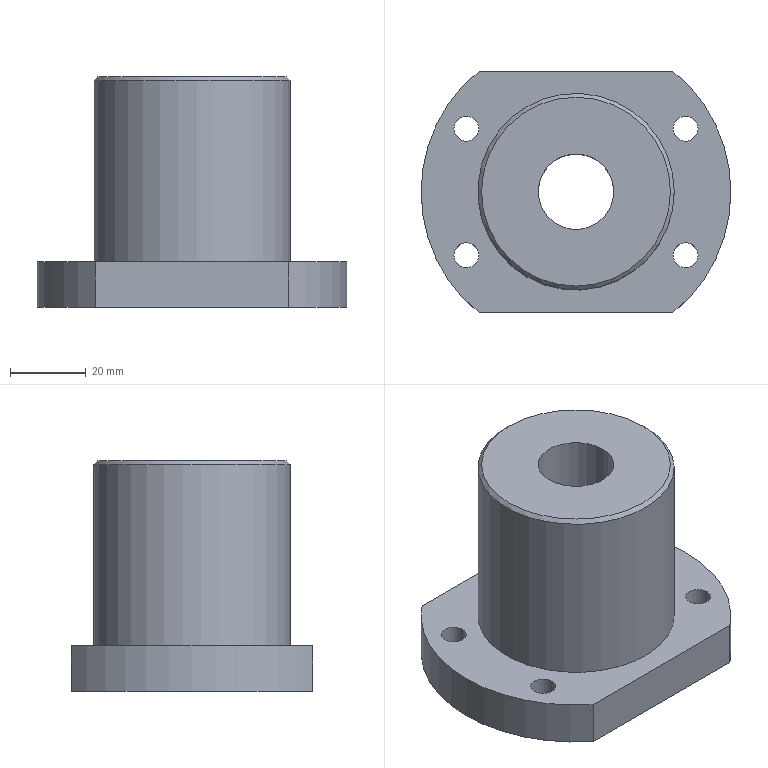Part | NX | 1 solid | 14 faces | box 82 x 64 x 61 mm | volume 138987 mm3 | cylinder 8 | plane 5 | cone 1 | commonest cylinder face diameters 6.6 x4 82 x2 20 x1 52 x1
STEP:
#1=CARTESIAN_POINT('',(32.312,16.75,12.));
#2=VERTEX_POINT('',#1);
#3=CARTESIAN_POINT('',(29.012,16.75,12.));
#4=DIRECTION('',(0.,0.,1.));
#5=DIRECTION('',(1.,0.,0.));
#6=AXIS2_PLACEMENT_3D('',#3,#4,#5);
#7=CIRCLE('',#6,3.3);
#8=EDGE_CURVE('',#2,#2,#7,.T.);
#9=ORIENTED_EDGE('',*,*,#8,.F.);
#10=EDGE_LOOP('',(#9));
#11=FACE_BOUND('',#10,.T.);
#12=CARTESIAN_POINT('',(-25.712,16.75,12.));
#13=VERTEX_POINT('',#12);
#14=CARTESIAN_POINT('',(-29.012,16.75,12.));
#15=DIRECTION('',(0.,0.,1.));
#16=DIRECTION('',(1.,0.,0.));
#17=AXIS2_PLACEMENT_3D('',#14,#15,#16);
#18=CIRCLE('',#17,3.3);
#19=EDGE_CURVE('',#13,#13,#18,.T.);
#20=ORIENTED_EDGE('',*,*,#19,.F.);
#21=EDGE_LOOP('',(#20));
#22=FACE_BOUND('',#21,.T.);
#23=CARTESIAN_POINT('',(32.312,-16.75,12.));
#24=VERTEX_POINT('',#23);
#25=CARTESIAN_POINT('',(29.012,-16.75,12.));
#26=DIRECTION('',(0.,0.,1.));
#27=DIRECTION('',(1.,0.,0.));
#28=AXIS2_PLACEMENT_3D('',#25,#26,#27);
#29=CIRCLE('',#28,3.3);
#30=EDGE_CURVE('',#24,#24,#29,.T.);
#31=ORIENTED_EDGE('',*,*,#30,.F.);
#32=EDGE_LOOP('',(#31));
#33=FACE_BOUND('',#32,.T.);
#34=CARTESIAN_POINT('',(-25.712,-16.75,12.));
#35=VERTEX_POINT('',#34);
#36=CARTESIAN_POINT('',(-29.012,-16.75,12.));
#37=DIRECTION('',(0.,0.,1.));
#38=DIRECTION('',(1.,0.,0.));
#39=AXIS2_PLACEMENT_3D('',#36,#37,#38);
#40=CIRCLE('',#39,3.3);
#41=EDGE_CURVE('',#35,#35,#40,.T.);
#42=ORIENTED_EDGE('',*,*,#41,.F.);
#43=EDGE_LOOP('',(#42));
#44=FACE_BOUND('',#43,.T.);
#45=CARTESIAN_POINT('',(26.,0.,12.));
#46=VERTEX_POINT('',#45);
#47=CARTESIAN_POINT('',(0.,0.,12.));
#48=DIRECTION('',(0.,0.,1.));
#49=DIRECTION('',(1.,0.,0.));
#50=AXIS2_PLACEMENT_3D('',#47,#48,#49);
#51=CIRCLE('',#50,26.);
#52=EDGE_CURVE('',#46,#46,#51,.T.);
#53=ORIENTED_EDGE('',*,*,#52,.F.);
#54=EDGE_LOOP('',(#53));
#55=FACE_BOUND('',#54,.T.);
#56=CARTESIAN_POINT('',(-25.632,32.,12.));
#57=VERTEX_POINT('',#56);
#58=CARTESIAN_POINT('',(-25.632,-32.,12.));
#59=VERTEX_POINT('',#58);
#60=CARTESIAN_POINT('',(0.,0.,12.));
#61=DIRECTION('',(0.,0.,1.));
#62=DIRECTION('',(1.,0.,0.));
#63=AXIS2_PLACEMENT_3D('',#60,#61,#62);
#64=CIRCLE('',#63,41.);
#65=EDGE_CURVE('',#57,#59,#64,.T.);
#66=ORIENTED_EDGE('',*,*,#65,.T.);
#67=CARTESIAN_POINT('',(25.632,-32.,12.));
#68=VERTEX_POINT('',#67);
#69=CARTESIAN_POINT('',(0.,-32.,12.));
#70=DIRECTION('',(1.,0.,0.));
#71=VECTOR('',#70,1000.);
#72=LINE('',#69,#71);
#73=EDGE_CURVE('',#59,#68,#72,.T.);
#74=ORIENTED_EDGE('',*,*,#73,.T.);
#75=CARTESIAN_POINT('',(25.632,32.,12.));
#76=VERTEX_POINT('',#75);
#77=CARTESIAN_POINT('',(0.,0.,12.));
#78=DIRECTION('',(0.,0.,1.));
#79=DIRECTION('',(1.,0.,0.));
#80=AXIS2_PLACEMENT_3D('',#77,#78,#79);
#81=CIRCLE('',#80,41.);
#82=EDGE_CURVE('',#68,#76,#81,.T.);
#83=ORIENTED_EDGE('',*,*,#82,.T.);
#84=CARTESIAN_POINT('',(0.,32.,12.));
#85=DIRECTION('',(-1.,0.,0.));
#86=VECTOR('',#85,1000.);
#87=LINE('',#84,#86);
#88=EDGE_CURVE('',#76,#57,#87,.T.);
#89=ORIENTED_EDGE('',*,*,#88,.T.);
#90=EDGE_LOOP('',(#66,#74,#83,#89));
#91=FACE_BOUND('',#90,.T.);
#92=CARTESIAN_POINT('',(0.,0.,12.));
#93=DIRECTION('',(0.,0.,1.));
#94=DIRECTION('',(1.,0.,0.));
#95=AXIS2_PLACEMENT_3D('',#92,#93,#94);
#96=PLANE('',#95);
#97=ADVANCED_FACE('',(#11,#22,#33,#44,#55,#91),#96,.T.);
#98=CARTESIAN_POINT('',(-25.632,-32.,0.));
#99=VERTEX_POINT('',#98);
#100=CARTESIAN_POINT('',(-25.632,-32.,12.));
#101=DIRECTION('',(0.,0.,-1.));
#102=VECTOR('',#101,1000.);
#103=LINE('',#100,#102);
#104=EDGE_CURVE('',#59,#99,#103,.T.);
#105=ORIENTED_EDGE('',*,*,#104,.F.);
#106=ORIENTED_EDGE('',*,*,#65,.F.);
#107=CARTESIAN_POINT('',(-25.632,32.,0.));
#108=VERTEX_POINT('',#107);
#109=CARTESIAN_POINT('',(-25.632,32.,12.));
#110=DIRECTION('',(0.,0.,-1.));
#111=VECTOR('',#110,1000.);
#112=LINE('',#109,#111);
#113=EDGE_CURVE('',#108,#57,#112,.F.);
#114=ORIENTED_EDGE('',*,*,#113,.F.);
#115=CARTESIAN_POINT('',(0.,0.,0.));
#116=DIRECTION('',(0.,0.,1.));
#117=DIRECTION('',(1.,0.,0.));
#118=AXIS2_PLACEMENT_3D('',#115,#116,#117);
#119=CIRCLE('',#118,41.);
#120=EDGE_CURVE('',#108,#99,#119,.T.);
#121=ORIENTED_EDGE('',*,*,#120,.T.);
#122=EDGE_LOOP('',(#105,#106,#114,#121));
#123=FACE_BOUND('',#122,.T.);
#124=CARTESIAN_POINT('',(0.,0.,12.));
#125=DIRECTION('',(0.,0.,-1.));
#126=DIRECTION('',(-1.,0.,0.));
#127=AXIS2_PLACEMENT_3D('',#124,#125,#126);
#128=CYLINDRICAL_SURFACE('',#127,41.);
#129=ADVANCED_FACE('',(#123),#128,.T.);
#130=CARTESIAN_POINT('',(25.632,-32.,0.));
#131=VERTEX_POINT('',#130);
#132=CARTESIAN_POINT('',(25.632,-32.,12.));
#133=DIRECTION('',(0.,0.,-1.));
#134=VECTOR('',#133,1000.);
#135=LINE('',#132,#134);
#136=EDGE_CURVE('',#131,#68,#135,.F.);
#137=ORIENTED_EDGE('',*,*,#136,.F.);
#138=CARTESIAN_POINT('',(25.632,32.,0.));
#139=VERTEX_POINT('',#138);
#140=CARTESIAN_POINT('',(0.,0.,0.));
#141=DIRECTION('',(0.,0.,1.));
#142=DIRECTION('',(1.,0.,0.));
#143=AXIS2_PLACEMENT_3D('',#140,#141,#142);
#144=CIRCLE('',#143,41.);
#145=EDGE_CURVE('',#131,#139,#144,.T.);
#146=ORIENTED_EDGE('',*,*,#145,.T.);
#147=CARTESIAN_POINT('',(25.632,32.,12.));
#148=DIRECTION('',(0.,0.,-1.));
#149=VECTOR('',#148,1000.);
#150=LINE('',#147,#149);
#151=EDGE_CURVE('',#76,#139,#150,.T.);
#152=ORIENTED_EDGE('',*,*,#151,.F.);
#153=ORIENTED_EDGE('',*,*,#82,.F.);
#154=EDGE_LOOP('',(#137,#146,#152,#153));
#155=FACE_BOUND('',#154,.T.);
#156=CARTESIAN_POINT('',(0.,0.,12.));
#157=DIRECTION('',(0.,0.,-1.));
#158=DIRECTION('',(-1.,0.,0.));
#159=AXIS2_PLACEMENT_3D('',#156,#157,#158);
#160=CYLINDRICAL_SURFACE('',#159,41.);
#161=ADVANCED_FACE('',(#155),#160,.T.);
#162=CARTESIAN_POINT('',(25.712,16.75,0.));
#163=VERTEX_POINT('',#162);
#164=CARTESIAN_POINT('',(29.012,16.75,0.));
#165=DIRECTION('',(0.,0.,-1.));
#166=DIRECTION('',(-1.,0.,0.));
#167=AXIS2_PLACEMENT_3D('',#164,#165,#166);
#168=CIRCLE('',#167,3.3);
#169=EDGE_CURVE('',#163,#163,#168,.T.);
#170=ORIENTED_EDGE('',*,*,#169,.F.);
#171=EDGE_LOOP('',(#170));
#172=FACE_BOUND('',#171,.T.);
#173=CARTESIAN_POINT('',(-32.312,16.75,0.));
#174=VERTEX_POINT('',#173);
#175=CARTESIAN_POINT('',(-29.012,16.75,0.));
#176=DIRECTION('',(0.,0.,-1.));
#177=DIRECTION('',(-1.,0.,0.));
#178=AXIS2_PLACEMENT_3D('',#175,#176,#177);
#179=CIRCLE('',#178,3.3);
#180=EDGE_CURVE('',#174,#174,#179,.T.);
#181=ORIENTED_EDGE('',*,*,#180,.F.);
#182=EDGE_LOOP('',(#181));
#183=FACE_BOUND('',#182,.T.);
#184=CARTESIAN_POINT('',(25.712,-16.75,0.));
#185=VERTEX_POINT('',#184);
#186=CARTESIAN_POINT('',(29.012,-16.75,0.));
#187=DIRECTION('',(0.,0.,-1.));
#188=DIRECTION('',(-1.,0.,0.));
#189=AXIS2_PLACEMENT_3D('',#186,#187,#188);
#190=CIRCLE('',#189,3.3);
#191=EDGE_CURVE('',#185,#185,#190,.T.);
#192=ORIENTED_EDGE('',*,*,#191,.F.);
#193=EDGE_LOOP('',(#192));
#194=FACE_BOUND('',#193,.T.);
#195=CARTESIAN_POINT('',(-32.312,-16.75,0.));
#196=VERTEX_POINT('',#195);
#197=CARTESIAN_POINT('',(-29.012,-16.75,0.));
#198=DIRECTION('',(0.,0.,-1.));
#199=DIRECTION('',(-1.,0.,0.));
#200=AXIS2_PLACEMENT_3D('',#197,#198,#199);
#201=CIRCLE('',#200,3.3);
#202=EDGE_CURVE('',#196,#196,#201,.T.);
#203=ORIENTED_EDGE('',*,*,#202,.F.);
#204=EDGE_LOOP('',(#203));
#205=FACE_BOUND('',#204,.T.);
#206=CARTESIAN_POINT('',(10.,0.,0.));
#207=VERTEX_POINT('',#206);
#208=CARTESIAN_POINT('',(0.,0.,0.));
#209=DIRECTION('',(0.,0.,1.));
#210=DIRECTION('',(1.,0.,0.));
#211=AXIS2_PLACEMENT_3D('',#208,#209,#210);
#212=CIRCLE('',#211,10.);
#213=EDGE_CURVE('',#207,#207,#212,.T.);
#214=ORIENTED_EDGE('',*,*,#213,.T.);
#215=EDGE_LOOP('',(#214));
#216=FACE_BOUND('',#215,.T.);
#217=CARTESIAN_POINT('',(0.,-32.,0.));
#218=DIRECTION('',(1.,0.,0.));
#219=VECTOR('',#218,1000.);
#220=LINE('',#217,#219);
#221=EDGE_CURVE('',#99,#131,#220,.T.);
#222=ORIENTED_EDGE('',*,*,#221,.F.);
#223=ORIENTED_EDGE('',*,*,#120,.F.);
#224=CARTESIAN_POINT('',(0.,32.,0.));
#225=DIRECTION('',(-1.,0.,0.));
#226=VECTOR('',#225,1000.);
#227=LINE('',#224,#226);
#228=EDGE_CURVE('',#139,#108,#227,.T.);
#229=ORIENTED_EDGE('',*,*,#228,.F.);
#230=ORIENTED_EDGE('',*,*,#145,.F.);
#231=EDGE_LOOP('',(#222,#223,#229,#230));
#232=FACE_BOUND('',#231,.T.);
#233=CARTESIAN_POINT('',(0.,0.,0.));
#234=DIRECTION('',(0.,0.,1.));
#235=DIRECTION('',(1.,0.,0.));
#236=AXIS2_PLACEMENT_3D('',#233,#234,#235);
#237=PLANE('',#236);
#238=ADVANCED_FACE('',(#172,#183,#194,#205,#216,#232),#237,.F.);
#239=CARTESIAN_POINT('',(26.,0.,60.));
#240=VERTEX_POINT('',#239);
#241=CARTESIAN_POINT('',(0.,0.,60.));
#242=DIRECTION('',(0.,0.,1.));
#243=DIRECTION('',(1.,0.,0.));
#244=AXIS2_PLACEMENT_3D('',#241,#242,#243);
#245=CIRCLE('',#244,26.);
#246=EDGE_CURVE('',#240,#240,#245,.F.);
#247=ORIENTED_EDGE('',*,*,#246,.T.);
#248=EDGE_LOOP('',(#247));
#249=FACE_BOUND('',#248,.T.);
#250=ORIENTED_EDGE('',*,*,#52,.T.);
#251=EDGE_LOOP('',(#250));
#252=FACE_BOUND('',#251,.T.);
#253=CARTESIAN_POINT('',(0.,0.,61.));
#254=DIRECTION('',(0.,0.,-1.));
#255=DIRECTION('',(-1.,0.,0.));
#256=AXIS2_PLACEMENT_3D('',#253,#254,#255);
#257=CYLINDRICAL_SURFACE('',#256,26.);
#258=ADVANCED_FACE('',(#249,#252),#257,.T.);
#259=CARTESIAN_POINT('',(25.,0.,61.));
#260=VERTEX_POINT('',#259);
#261=CARTESIAN_POINT('',(0.,0.,61.));
#262=DIRECTION('',(0.,0.,1.));
#263=DIRECTION('',(1.,0.,0.));
#264=AXIS2_PLACEMENT_3D('',#261,#262,#263);
#265=CIRCLE('',#264,25.);
#266=EDGE_CURVE('',#260,#260,#265,.T.);
#267=ORIENTED_EDGE('',*,*,#266,.T.);
#268=EDGE_LOOP('',(#267));
#269=FACE_BOUND('',#268,.T.);
#270=CARTESIAN_POINT('',(10.,0.,61.));
#271=VERTEX_POINT('',#270);
#272=CARTESIAN_POINT('',(0.,0.,61.));
#273=DIRECTION('',(0.,0.,1.));
#274=DIRECTION('',(1.,0.,0.));
#275=AXIS2_PLACEMENT_3D('',#272,#273,#274);
#276=CIRCLE('',#275,10.);
#277=EDGE_CURVE('',#271,#271,#276,.T.);
#278=ORIENTED_EDGE('',*,*,#277,.F.);
#279=EDGE_LOOP('',(#278));
#280=FACE_BOUND('',#279,.T.);
#281=CARTESIAN_POINT('',(0.,0.,61.));
#282=DIRECTION('',(0.,0.,1.));
#283=DIRECTION('',(1.,0.,0.));
#284=AXIS2_PLACEMENT_3D('',#281,#282,#283);
#285=PLANE('',#284);
#286=ADVANCED_FACE('',(#269,#280),#285,.T.);
#287=ORIENTED_EDGE('',*,*,#213,.F.);
#288=EDGE_LOOP('',(#287));
#289=FACE_BOUND('',#288,.T.);
#290=ORIENTED_EDGE('',*,*,#277,.T.);
#291=EDGE_LOOP('',(#290));
#292=FACE_BOUND('',#291,.T.);
#293=CARTESIAN_POINT('',(0.,0.,0.));
#294=DIRECTION('',(0.,0.,1.));
#295=DIRECTION('',(1.,0.,0.));
#296=AXIS2_PLACEMENT_3D('',#293,#294,#295);
#297=CYLINDRICAL_SURFACE('',#296,10.);
#298=ADVANCED_FACE('',(#289,#292),#297,.F.);
#299=ORIENTED_EDGE('',*,*,#151,.T.);
#300=ORIENTED_EDGE('',*,*,#228,.T.);
#301=ORIENTED_EDGE('',*,*,#113,.T.);
#302=ORIENTED_EDGE('',*,*,#88,.F.);
#303=EDGE_LOOP('',(#299,#300,#301,#302));
#304=FACE_BOUND('',#303,.T.);
#305=CARTESIAN_POINT('',(50.,32.,37.));
#306=DIRECTION('',(0.,1.,0.));
#307=DIRECTION('',(0.,0.,1.));
#308=AXIS2_PLACEMENT_3D('',#305,#306,#307);
#309=PLANE('',#308);
#310=ADVANCED_FACE('',(#304),#309,.T.);
#311=ORIENTED_EDGE('',*,*,#104,.T.);
#312=ORIENTED_EDGE('',*,*,#221,.T.);
#313=ORIENTED_EDGE('',*,*,#136,.T.);
#314=ORIENTED_EDGE('',*,*,#73,.F.);
#315=EDGE_LOOP('',(#311,#312,#313,#314));
#316=FACE_BOUND('',#315,.T.);
#317=CARTESIAN_POINT('',(50.,-32.,37.));
#318=DIRECTION('',(0.,-1.,0.));
#319=DIRECTION('',(0.,0.,-1.));
#320=AXIS2_PLACEMENT_3D('',#317,#318,#319);
#321=PLANE('',#320);
#322=ADVANCED_FACE('',(#316),#321,.T.);
#323=ORIENTED_EDGE('',*,*,#246,.F.);
#324=EDGE_LOOP('',(#323));
#325=FACE_BOUND('',#324,.T.);
#326=ORIENTED_EDGE('',*,*,#266,.F.);
#327=EDGE_LOOP('',(#326));
#328=FACE_BOUND('',#327,.T.);
#329=CARTESIAN_POINT('',(0.,0.,61.));
#330=DIRECTION('',(0.,0.,-1.));
#331=DIRECTION('',(-1.,0.,0.));
#332=AXIS2_PLACEMENT_3D('',#329,#330,#331);
#333=CONICAL_SURFACE('',#332,25.,0.7854);
#334=ADVANCED_FACE('',(#325,#328),#333,.T.);
#335=ORIENTED_EDGE('',*,*,#41,.T.);
#336=EDGE_LOOP('',(#335));
#337=FACE_BOUND('',#336,.T.);
#338=ORIENTED_EDGE('',*,*,#202,.T.);
#339=EDGE_LOOP('',(#338));
#340=FACE_BOUND('',#339,.T.);
#341=CARTESIAN_POINT('',(-29.012,-16.75,0.));
#342=DIRECTION('',(0.,0.,-1.));
#343=DIRECTION('',(-1.,0.,0.));
#344=AXIS2_PLACEMENT_3D('',#341,#342,#343);
#345=CYLINDRICAL_SURFACE('',#344,3.3);
#346=ADVANCED_FACE('',(#337,#340),#345,.F.);
#347=ORIENTED_EDGE('',*,*,#30,.T.);
#348=EDGE_LOOP('',(#347));
#349=FACE_BOUND('',#348,.T.);
#350=ORIENTED_EDGE('',*,*,#191,.T.);
#351=EDGE_LOOP('',(#350));
#352=FACE_BOUND('',#351,.T.);
#353=CARTESIAN_POINT('',(29.012,-16.75,0.));
#354=DIRECTION('',(0.,0.,-1.));
#355=DIRECTION('',(-1.,0.,0.));
#356=AXIS2_PLACEMENT_3D('',#353,#354,#355);
#357=CYLINDRICAL_SURFACE('',#356,3.3);
#358=ADVANCED_FACE('',(#349,#352),#357,.F.);
#359=ORIENTED_EDGE('',*,*,#19,.T.);
#360=EDGE_LOOP('',(#359));
#361=FACE_BOUND('',#360,.T.);
#362=ORIENTED_EDGE('',*,*,#180,.T.);
#363=EDGE_LOOP('',(#362));
#364=FACE_BOUND('',#363,.T.);
#365=CARTESIAN_POINT('',(-29.012,16.75,0.));
#366=DIRECTION('',(0.,0.,-1.));
#367=DIRECTION('',(-1.,0.,0.));
#368=AXIS2_PLACEMENT_3D('',#365,#366,#367);
#369=CYLINDRICAL_SURFACE('',#368,3.3);
#370=ADVANCED_FACE('',(#361,#364),#369,.F.);
#371=ORIENTED_EDGE('',*,*,#8,.T.);
#372=EDGE_LOOP('',(#371));
#373=FACE_BOUND('',#372,.T.);
#374=ORIENTED_EDGE('',*,*,#169,.T.);
#375=EDGE_LOOP('',(#374));
#376=FACE_BOUND('',#375,.T.);
#377=CARTESIAN_POINT('',(29.012,16.75,0.));
#378=DIRECTION('',(0.,0.,-1.));
#379=DIRECTION('',(-1.,0.,0.));
#380=AXIS2_PLACEMENT_3D('',#377,#378,#379);
#381=CYLINDRICAL_SURFACE('',#380,3.3);
#382=ADVANCED_FACE('',(#373,#376),#381,.F.);
#383=CLOSED_SHELL('',(#97,#129,#161,#238,#258,#286,#298,#310,#322,#334,#346,#358,#370,#382));
#384=MANIFOLD_SOLID_BREP('',#383);
#385=(LENGTH_UNIT()NAMED_UNIT(*)SI_UNIT(.MILLI.,.METRE.));
#386=UNCERTAINTY_MEASURE_WITH_UNIT(LENGTH_MEASURE(0.00001),#385,'','');
#387=(NAMED_UNIT(*)PLANE_ANGLE_UNIT()SI_UNIT($,.RADIAN.));
#388=(NAMED_UNIT(*)SI_UNIT($,.STERADIAN.)SOLID_ANGLE_UNIT());
#389=(GEOMETRIC_REPRESENTATION_CONTEXT(3)GLOBAL_UNCERTAINTY_ASSIGNED_CONTEXT((#386))GLOBAL_UNIT_ASSIGNED_CONTEXT((#385,#387,#388))REPRESENTATION_CONTEXT('',''));
#390=ADVANCED_BREP_SHAPE_REPRESENTATION('',(#384),#389);